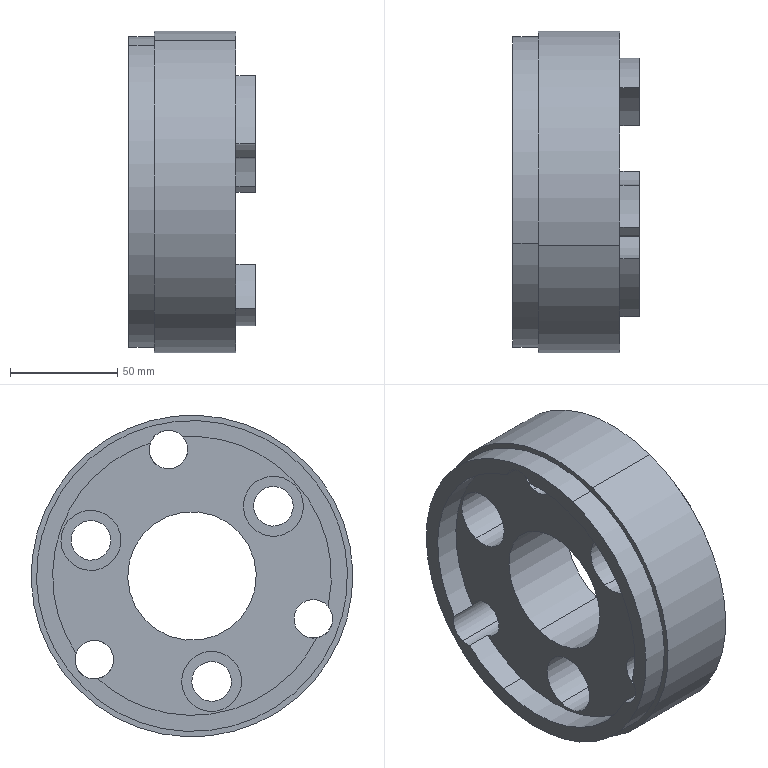Part | NX | features BREP 1 | 1 solid | 51 faces | box 59 x 150 x 150 mm | volume 529858 mm3 | cylinder 41 | plane 10 | commonest cylinder face diameters 18 x6 18.5 x6 28 x6 85 x6 130 x5 75 x3